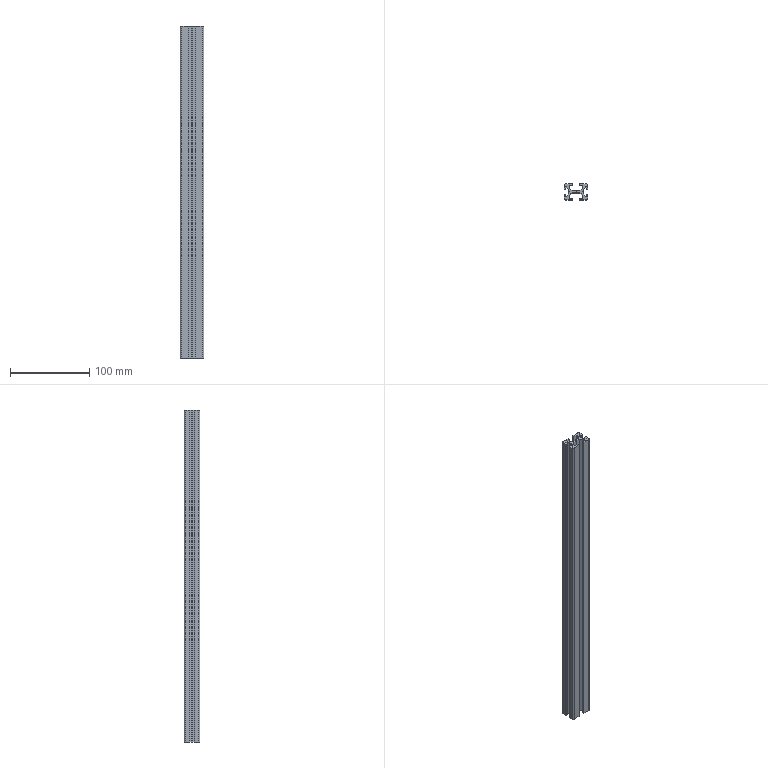Part | STEP file | 11-XHFS6-5Y-2030-31511 | 1 solid | 70 faces | box 30 x 20 x 420 mm | volume 106427 mm3 | plane 58 | cylinder 12 | commonest cylinder face diameters 0.6 x8 4 x4